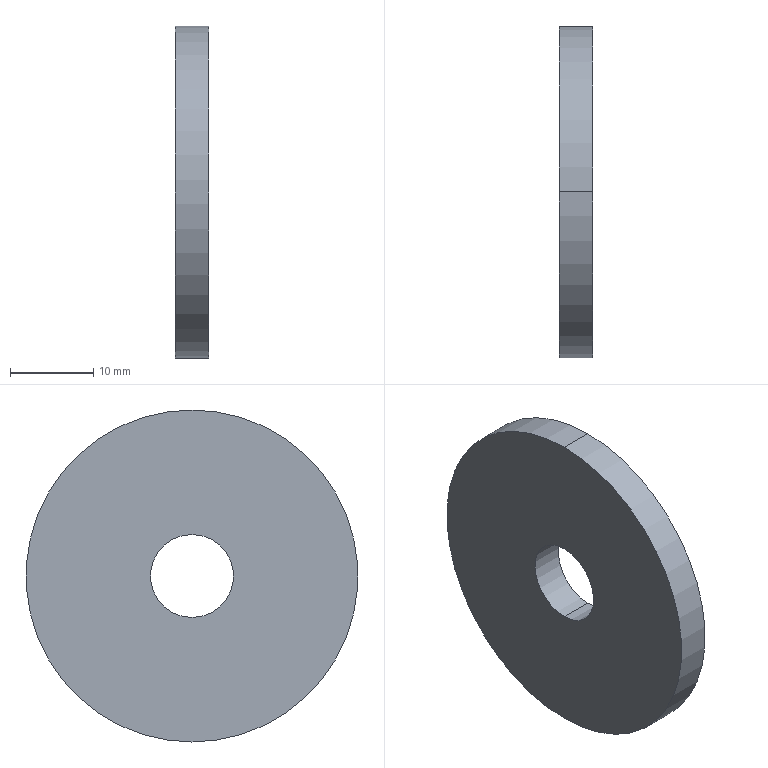Part | SolidWorks | features Extrusion 1 | 1 solid | 6 faces | box 4 x 40 x 40 mm | volume 4712 mm3 | cylinder 4 | plane 2 | commonest cylinder face diameters 10 x2 40 x2
STEP:
#1=CARTESIAN_POINT('',(2.,0.,5.));
#2=VERTEX_POINT('',#1);
#3=CARTESIAN_POINT('',(2.,0.,-5.));
#4=VERTEX_POINT('',#3);
#5=CARTESIAN_POINT('',(2.,0.,0.));
#6=DIRECTION('',(1.,0.,0.));
#7=DIRECTION('',(0.,0.,-1.));
#8=AXIS2_PLACEMENT_3D('',#5,#6,#7);
#9=CIRCLE('',#8,5.);
#10=EDGE_CURVE('',#2,#4,#9,.T.);
#11=ORIENTED_EDGE('',*,*,#10,.T.);
#12=CARTESIAN_POINT('',(-2.,0.,-5.));
#13=VERTEX_POINT('',#12);
#14=CARTESIAN_POINT('',(2.,0.,-5.));
#15=DIRECTION('',(-1.,0.,0.));
#16=VECTOR('',#15,1000.);
#17=LINE('',#14,#16);
#18=EDGE_CURVE('',#4,#13,#17,.T.);
#19=ORIENTED_EDGE('',*,*,#18,.T.);
#20=CARTESIAN_POINT('',(-2.,0.,5.));
#21=VERTEX_POINT('',#20);
#22=CARTESIAN_POINT('',(-2.,0.,0.));
#23=DIRECTION('',(1.,0.,0.));
#24=DIRECTION('',(0.,0.,-1.));
#25=AXIS2_PLACEMENT_3D('',#22,#23,#24);
#26=CIRCLE('',#25,5.);
#27=EDGE_CURVE('',#21,#13,#26,.T.);
#28=ORIENTED_EDGE('',*,*,#27,.F.);
#29=CARTESIAN_POINT('',(2.,0.,5.));
#30=DIRECTION('',(-1.,0.,0.));
#31=VECTOR('',#30,1000.);
#32=LINE('',#29,#31);
#33=EDGE_CURVE('',#2,#21,#32,.T.);
#34=ORIENTED_EDGE('',*,*,#33,.F.);
#35=EDGE_LOOP('',(#11,#19,#28,#34));
#36=FACE_OUTER_BOUND('',#35,.T.);
#37=CARTESIAN_POINT('',(2.,0.,0.));
#38=DIRECTION('',(-1.,0.,0.));
#39=DIRECTION('',(0.,0.,1.));
#40=AXIS2_PLACEMENT_3D('',#37,#38,#39);
#41=CYLINDRICAL_SURFACE('',#40,5.);
#42=ADVANCED_FACE('',(#36),#41,.F.);
#43=CARTESIAN_POINT('',(2.,0.,-20.));
#44=VERTEX_POINT('',#43);
#45=CARTESIAN_POINT('',(2.,0.,20.));
#46=VERTEX_POINT('',#45);
#47=CARTESIAN_POINT('',(2.,0.,0.));
#48=DIRECTION('',(1.,0.,0.));
#49=DIRECTION('',(0.,0.,-1.));
#50=AXIS2_PLACEMENT_3D('',#47,#48,#49);
#51=CIRCLE('',#50,20.);
#52=EDGE_CURVE('',#44,#46,#51,.T.);
#53=ORIENTED_EDGE('',*,*,#52,.F.);
#54=CARTESIAN_POINT('',(-2.,0.,-20.));
#55=VERTEX_POINT('',#54);
#56=CARTESIAN_POINT('',(2.,0.,-20.));
#57=DIRECTION('',(-1.,0.,0.));
#58=VECTOR('',#57,1000.);
#59=LINE('',#56,#58);
#60=EDGE_CURVE('',#44,#55,#59,.T.);
#61=ORIENTED_EDGE('',*,*,#60,.T.);
#62=CARTESIAN_POINT('',(-2.,0.,20.));
#63=VERTEX_POINT('',#62);
#64=CARTESIAN_POINT('',(-2.,0.,0.));
#65=DIRECTION('',(1.,0.,0.));
#66=DIRECTION('',(0.,0.,-1.));
#67=AXIS2_PLACEMENT_3D('',#64,#65,#66);
#68=CIRCLE('',#67,20.);
#69=EDGE_CURVE('',#55,#63,#68,.T.);
#70=ORIENTED_EDGE('',*,*,#69,.T.);
#71=CARTESIAN_POINT('',(2.,0.,20.));
#72=DIRECTION('',(-1.,0.,0.));
#73=VECTOR('',#72,1000.);
#74=LINE('',#71,#73);
#75=EDGE_CURVE('',#46,#63,#74,.T.);
#76=ORIENTED_EDGE('',*,*,#75,.F.);
#77=EDGE_LOOP('',(#53,#61,#70,#76));
#78=FACE_OUTER_BOUND('',#77,.T.);
#79=CARTESIAN_POINT('',(2.,0.,0.));
#80=DIRECTION('',(-1.,0.,0.));
#81=DIRECTION('',(0.,0.,1.));
#82=AXIS2_PLACEMENT_3D('',#79,#80,#81);
#83=CYLINDRICAL_SURFACE('',#82,20.);
#84=ADVANCED_FACE('',(#78),#83,.T.);
#85=CARTESIAN_POINT('',(2.,0.,0.));
#86=DIRECTION('',(1.,0.,0.));
#87=DIRECTION('',(0.,0.,-1.));
#88=AXIS2_PLACEMENT_3D('',#85,#86,#87);
#89=CIRCLE('',#88,20.);
#90=EDGE_CURVE('',#46,#44,#89,.T.);
#91=ORIENTED_EDGE('',*,*,#90,.T.);
#92=ORIENTED_EDGE('',*,*,#52,.T.);
#93=EDGE_LOOP('',(#91,#92));
#94=FACE_OUTER_BOUND('',#93,.T.);
#95=ORIENTED_EDGE('',*,*,#10,.F.);
#96=CARTESIAN_POINT('',(2.,0.,0.));
#97=DIRECTION('',(1.,0.,0.));
#98=DIRECTION('',(0.,0.,-1.));
#99=AXIS2_PLACEMENT_3D('',#96,#97,#98);
#100=CIRCLE('',#99,5.);
#101=EDGE_CURVE('',#4,#2,#100,.T.);
#102=ORIENTED_EDGE('',*,*,#101,.F.);
#103=EDGE_LOOP('',(#95,#102));
#104=FACE_BOUND('',#103,.T.);
#105=CARTESIAN_POINT('',(2.,0.,0.));
#106=DIRECTION('',(1.,0.,0.));
#107=DIRECTION('',(0.,0.,-1.));
#108=AXIS2_PLACEMENT_3D('',#105,#106,#107);
#109=PLANE('',#108);
#110=ADVANCED_FACE('',(#94,#104),#109,.T.);
#111=CARTESIAN_POINT('',(-2.,0.,0.));
#112=DIRECTION('',(1.,0.,0.));
#113=DIRECTION('',(0.,0.,-1.));
#114=AXIS2_PLACEMENT_3D('',#111,#112,#113);
#115=CIRCLE('',#114,20.);
#116=EDGE_CURVE('',#63,#55,#115,.T.);
#117=ORIENTED_EDGE('',*,*,#116,.F.);
#118=ORIENTED_EDGE('',*,*,#69,.F.);
#119=EDGE_LOOP('',(#117,#118));
#120=FACE_OUTER_BOUND('',#119,.T.);
#121=ORIENTED_EDGE('',*,*,#27,.T.);
#122=CARTESIAN_POINT('',(-2.,0.,0.));
#123=DIRECTION('',(1.,0.,0.));
#124=DIRECTION('',(0.,0.,-1.));
#125=AXIS2_PLACEMENT_3D('',#122,#123,#124);
#126=CIRCLE('',#125,5.);
#127=EDGE_CURVE('',#13,#21,#126,.T.);
#128=ORIENTED_EDGE('',*,*,#127,.T.);
#129=EDGE_LOOP('',(#121,#128));
#130=FACE_BOUND('',#129,.T.);
#131=CARTESIAN_POINT('',(-2.,0.,0.));
#132=DIRECTION('',(1.,0.,0.));
#133=DIRECTION('',(0.,0.,-1.));
#134=AXIS2_PLACEMENT_3D('',#131,#132,#133);
#135=PLANE('',#134);
#136=ADVANCED_FACE('',(#120,#130),#135,.F.);
#137=ORIENTED_EDGE('',*,*,#60,.F.);
#138=ORIENTED_EDGE('',*,*,#90,.F.);
#139=ORIENTED_EDGE('',*,*,#75,.T.);
#140=ORIENTED_EDGE('',*,*,#116,.T.);
#141=EDGE_LOOP('',(#137,#138,#139,#140));
#142=FACE_OUTER_BOUND('',#141,.T.);
#143=CARTESIAN_POINT('',(2.,0.,0.));
#144=DIRECTION('',(-1.,0.,0.));
#145=DIRECTION('',(0.,0.,1.));
#146=AXIS2_PLACEMENT_3D('',#143,#144,#145);
#147=CYLINDRICAL_SURFACE('',#146,20.);
#148=ADVANCED_FACE('',(#142),#147,.T.);
#149=ORIENTED_EDGE('',*,*,#18,.F.);
#150=ORIENTED_EDGE('',*,*,#101,.T.);
#151=ORIENTED_EDGE('',*,*,#33,.T.);
#152=ORIENTED_EDGE('',*,*,#127,.F.);
#153=EDGE_LOOP('',(#149,#150,#151,#152));
#154=FACE_OUTER_BOUND('',#153,.T.);
#155=CARTESIAN_POINT('',(2.,0.,0.));
#156=DIRECTION('',(-1.,0.,0.));
#157=DIRECTION('',(0.,0.,1.));
#158=AXIS2_PLACEMENT_3D('',#155,#156,#157);
#159=CYLINDRICAL_SURFACE('',#158,5.);
#160=ADVANCED_FACE('',(#154),#159,.F.);
#161=CLOSED_SHELL('',(#42,#84,#110,#136,#148,#160));
#162=MANIFOLD_SOLID_BREP('',#161);
#163=CARTESIAN_POINT('',(0.,0.,0.));
#164=DIRECTION('',(0.,0.,1.));
#165=DIRECTION('',(1.,0.,0.));
#166=AXIS2_PLACEMENT_3D('',#163,#164,#165);
#167=(LENGTH_UNIT()NAMED_UNIT(*)SI_UNIT(.MILLI.,.METRE.));
#168=UNCERTAINTY_MEASURE_WITH_UNIT(LENGTH_MEASURE(0.00001),#167,'','');
#169=(NAMED_UNIT(*)PLANE_ANGLE_UNIT()SI_UNIT($,.RADIAN.));
#170=(NAMED_UNIT(*)SI_UNIT($,.STERADIAN.)SOLID_ANGLE_UNIT());
#171=(GEOMETRIC_REPRESENTATION_CONTEXT(3)GLOBAL_UNCERTAINTY_ASSIGNED_CONTEXT((#168))GLOBAL_UNIT_ASSIGNED_CONTEXT((#167,#169,#170))REPRESENTATION_CONTEXT('',''));
#172=ADVANCED_BREP_SHAPE_REPRESENTATION('',(#162,#166),#171);